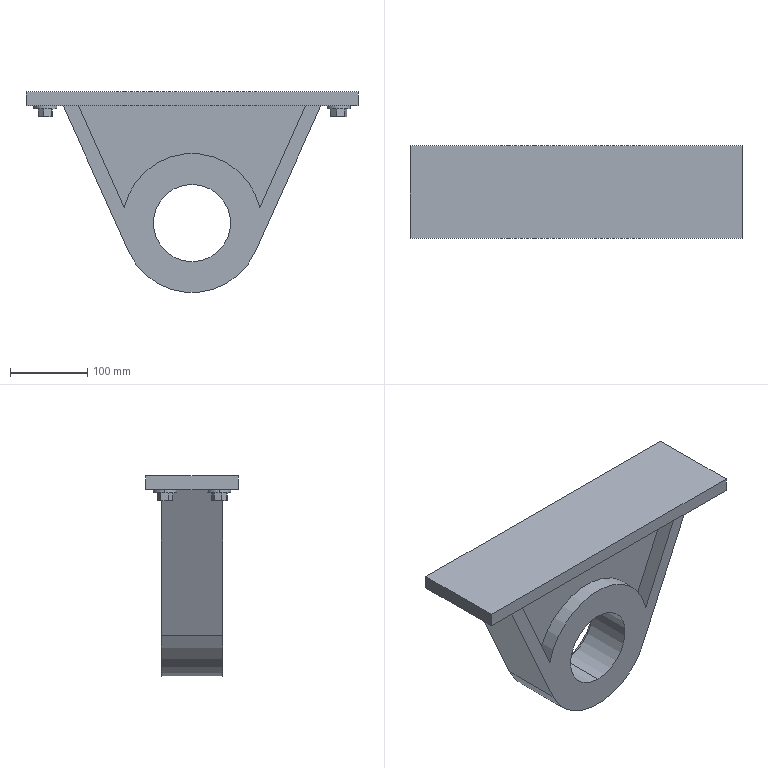Part | SolidWorks | features ICE 5, Extrusion 1, MirrorPattern 1 | 1 solid | 65 faces | box 430 x 120 x 260 mm | volume 3516427 mm3 | plane 49 | cylinder 16 | commonest cylinder face diameters 30 x8 180 x4 100 x2 150 x2